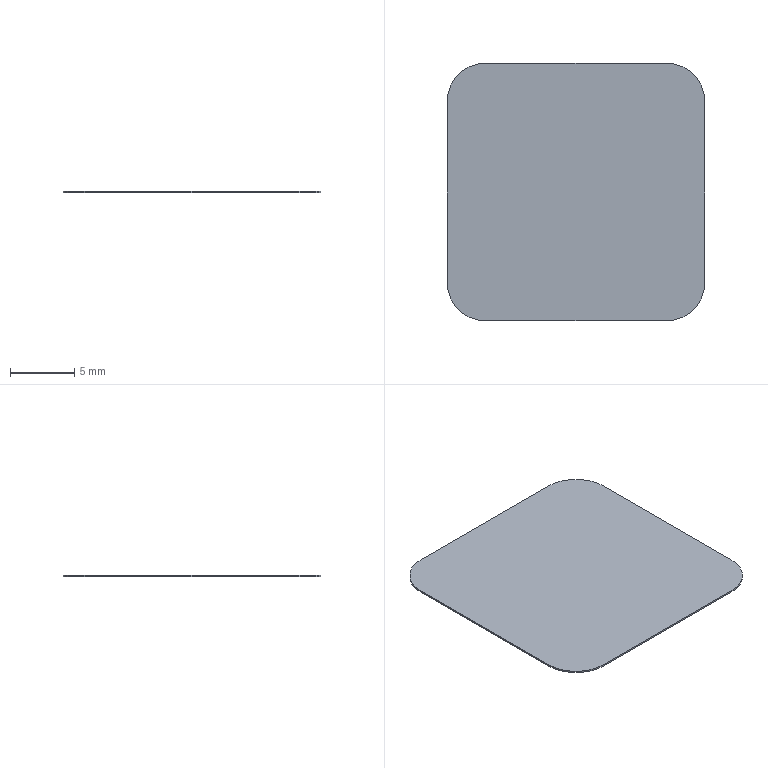Part | STEP file | 68423252 | 1 solid | 10 faces | box 20 x 20 x 0.125 mm | volume 49.034 mm3 | plane 6 | cylinder 4 | commonest cylinder face diameters 6 x4
STEP:
#1=CARTESIAN_POINT('',(0.,0.,0.));
#2=DIRECTION('',(0.,0.,1.));
#3=DIRECTION('',(1.,0.,0.));
#4=AXIS2_PLACEMENT_3D('',#1,#2,#3);
#5=CARTESIAN_POINT('',(-10.,17.,0.));
#6=VERTEX_POINT('',#5);
#7=CARTESIAN_POINT('',(-7.,20.,0.));
#8=VERTEX_POINT('',#7);
#9=CARTESIAN_POINT('',(-7.,17.,0.));
#10=DIRECTION('',(0.,0.,-1.));
#11=DIRECTION('',(-1.,0.,0.));
#12=AXIS2_PLACEMENT_3D('',#9,#10,#11);
#13=CIRCLE('',#12,3.);
#14=CARTESIAN_POINT('',(0.,0.,0.));
#15=DIRECTION('',(0.,0.,1.));
#16=DIRECTION('',(1.,0.,0.));
#17=AXIS2_PLACEMENT_3D('',#14,#15,#16);
#18=PLANE('',#17);
#19=CARTESIAN_POINT('',(-10.,17.));
#20=CARTESIAN_POINT('',(-10.,22.196));
#21=CARTESIAN_POINT('',(-5.5,19.598));
#22=CARTESIAN_POINT('',(-1.,17.));
#23=CARTESIAN_POINT('',(-5.5,14.402));
#24=CARTESIAN_POINT('',(-10.,11.804));
#25=CARTESIAN_POINT('',(-10.,17.));
#26=(BOUNDED_CURVE()B_SPLINE_CURVE(2,(#19,#20,#21,#22,#23,#24,#25),.UNSPECIFIED.,.T.,.F.)B_SPLINE_CURVE_WITH_KNOTS((1,2,2,2,2,1),(-2.094,0.,2.094,4.189,6.283,8.378),.UNSPECIFIED.)CURVE()GEOMETRIC_REPRESENTATION_ITEM()RATIONAL_B_SPLINE_CURVE((1.,0.5,1.,0.5,1.,0.5,1.))REPRESENTATION_ITEM(''));
#27=(GEOMETRIC_REPRESENTATION_CONTEXT(2)PARAMETRIC_REPRESENTATION_CONTEXT()REPRESENTATION_CONTEXT('',''));
#28=DEFINITIONAL_REPRESENTATION('',(#26),#27);
#29=PCURVE('',#18,#28);
#30=CARTESIAN_POINT('',(-7.,17.,0.202));
#31=DIRECTION('',(0.,0.,-1.));
#32=DIRECTION('',(-1.,0.,0.));
#33=AXIS2_PLACEMENT_3D('',#30,#31,#32);
#34=CYLINDRICAL_SURFACE('',#33,3.);
#35=CARTESIAN_POINT('',(0.,0.202));
#36=DIRECTION('',(1.,0.));
#37=VECTOR('',#36,1.);
#38=LINE('',#35,#37);
#39=(GEOMETRIC_REPRESENTATION_CONTEXT(2)PARAMETRIC_REPRESENTATION_CONTEXT()REPRESENTATION_CONTEXT('',''));
#40=DEFINITIONAL_REPRESENTATION('',(#38),#39);
#41=PCURVE('',#34,#40);
#42=SURFACE_CURVE('',#13,(#29,#41),.PCURVE_S1.);
#43=EDGE_CURVE('',#6,#8,#42,.T.);
#44=ORIENTED_EDGE('',*,*,#43,.F.);
#45=CARTESIAN_POINT('',(-10.,3.,0.));
#46=VERTEX_POINT('',#45);
#47=CARTESIAN_POINT('',(-10.,17.,0.));
#48=DIRECTION('',(0.,-1.,0.));
#49=VECTOR('',#48,1.);
#50=LINE('',#47,#49);
#51=CARTESIAN_POINT('',(-10.,17.));
#52=DIRECTION('',(0.,-1.));
#53=VECTOR('',#52,1.);
#54=LINE('',#51,#53);
#55=(GEOMETRIC_REPRESENTATION_CONTEXT(2)PARAMETRIC_REPRESENTATION_CONTEXT()REPRESENTATION_CONTEXT('',''));
#56=DEFINITIONAL_REPRESENTATION('',(#54),#55);
#57=PCURVE('',#18,#56);
#58=CARTESIAN_POINT('',(-10.,20.,0.));
#59=DIRECTION('',(-1.,0.,0.));
#60=DIRECTION('',(0.,-1.,0.));
#61=AXIS2_PLACEMENT_3D('',#58,#59,#60);
#62=PLANE('',#61);
#63=CARTESIAN_POINT('',(3.,0.));
#64=DIRECTION('',(1.,0.));
#65=VECTOR('',#64,1.);
#66=LINE('',#63,#65);
#67=(GEOMETRIC_REPRESENTATION_CONTEXT(2)PARAMETRIC_REPRESENTATION_CONTEXT()REPRESENTATION_CONTEXT('',''));
#68=DEFINITIONAL_REPRESENTATION('',(#66),#67);
#69=PCURVE('',#62,#68);
#70=SURFACE_CURVE('',#50,(#57,#69),.PCURVE_S1.);
#71=EDGE_CURVE('',#6,#46,#70,.T.);
#72=ORIENTED_EDGE('',*,*,#71,.T.);
#73=CARTESIAN_POINT('',(-7.,0.,0.));
#74=VERTEX_POINT('',#73);
#75=CARTESIAN_POINT('',(-7.,3.,0.));
#76=DIRECTION('',(0.,0.,-1.));
#77=DIRECTION('',(0.,-1.,0.));
#78=AXIS2_PLACEMENT_3D('',#75,#76,#77);
#79=CIRCLE('',#78,3.);
#80=CARTESIAN_POINT('',(-7.,0.));
#81=CARTESIAN_POINT('',(-12.196,0.));
#82=CARTESIAN_POINT('',(-9.598,4.5));
#83=CARTESIAN_POINT('',(-7.,9.));
#84=CARTESIAN_POINT('',(-4.402,4.5));
#85=CARTESIAN_POINT('',(-1.804,0.));
#86=CARTESIAN_POINT('',(-7.,0.));
#87=(BOUNDED_CURVE()B_SPLINE_CURVE(2,(#80,#81,#82,#83,#84,#85,#86),.UNSPECIFIED.,.T.,.F.)B_SPLINE_CURVE_WITH_KNOTS((1,2,2,2,2,1),(-2.094,0.,2.094,4.189,6.283,8.378),.UNSPECIFIED.)CURVE()GEOMETRIC_REPRESENTATION_ITEM()RATIONAL_B_SPLINE_CURVE((1.,0.5,1.,0.5,1.,0.5,1.))REPRESENTATION_ITEM(''));
#88=(GEOMETRIC_REPRESENTATION_CONTEXT(2)PARAMETRIC_REPRESENTATION_CONTEXT()REPRESENTATION_CONTEXT('',''));
#89=DEFINITIONAL_REPRESENTATION('',(#87),#88);
#90=PCURVE('',#18,#89);
#91=CARTESIAN_POINT('',(-7.,3.,-0.06577));
#92=DIRECTION('',(0.,0.,1.));
#93=DIRECTION('',(-1.,0.,0.));
#94=AXIS2_PLACEMENT_3D('',#91,#92,#93);
#95=CYLINDRICAL_SURFACE('',#94,3.);
#96=CARTESIAN_POINT('',(1.571,0.06577));
#97=DIRECTION('',(-1.,0.));
#98=VECTOR('',#97,1.);
#99=LINE('',#96,#98);
#100=(GEOMETRIC_REPRESENTATION_CONTEXT(2)PARAMETRIC_REPRESENTATION_CONTEXT()REPRESENTATION_CONTEXT('',''));
#101=DEFINITIONAL_REPRESENTATION('',(#99),#100);
#102=PCURVE('',#95,#101);
#103=SURFACE_CURVE('',#79,(#90,#102),.PCURVE_S1.);
#104=EDGE_CURVE('',#74,#46,#103,.T.);
#105=ORIENTED_EDGE('',*,*,#104,.F.);
#106=CARTESIAN_POINT('',(7.,0.,0.));
#107=VERTEX_POINT('',#106);
#108=CARTESIAN_POINT('',(-7.,0.,0.));
#109=DIRECTION('',(1.,0.,0.));
#110=VECTOR('',#109,1.);
#111=LINE('',#108,#110);
#112=CARTESIAN_POINT('',(-7.,0.));
#113=DIRECTION('',(1.,0.));
#114=VECTOR('',#113,1.);
#115=LINE('',#112,#114);
#116=(GEOMETRIC_REPRESENTATION_CONTEXT(2)PARAMETRIC_REPRESENTATION_CONTEXT()REPRESENTATION_CONTEXT('',''));
#117=DEFINITIONAL_REPRESENTATION('',(#115),#116);
#118=PCURVE('',#18,#117);
#119=CARTESIAN_POINT('',(10.,0.,0.125));
#120=DIRECTION('',(0.,1.,0.));
#121=DIRECTION('',(-1.,0.,0.));
#122=AXIS2_PLACEMENT_3D('',#119,#120,#121);
#123=PLANE('',#122);
#124=CARTESIAN_POINT('',(17.,-0.125));
#125=DIRECTION('',(-1.,0.));
#126=VECTOR('',#125,1.);
#127=LINE('',#124,#126);
#128=(GEOMETRIC_REPRESENTATION_CONTEXT(2)PARAMETRIC_REPRESENTATION_CONTEXT()REPRESENTATION_CONTEXT('',''));
#129=DEFINITIONAL_REPRESENTATION('',(#127),#128);
#130=PCURVE('',#123,#129);
#131=SURFACE_CURVE('',#111,(#118,#130),.PCURVE_S1.);
#132=EDGE_CURVE('',#74,#107,#131,.T.);
#133=ORIENTED_EDGE('',*,*,#132,.T.);
#134=CARTESIAN_POINT('',(10.,3.,0.));
#135=VERTEX_POINT('',#134);
#136=CARTESIAN_POINT('',(7.,3.,0.));
#137=DIRECTION('',(0.,0.,-1.));
#138=DIRECTION('',(1.,0.,0.));
#139=AXIS2_PLACEMENT_3D('',#136,#137,#138);
#140=CIRCLE('',#139,3.);
#141=CARTESIAN_POINT('',(10.,3.));
#142=CARTESIAN_POINT('',(10.,-2.196));
#143=CARTESIAN_POINT('',(5.5,0.4019));
#144=CARTESIAN_POINT('',(1.,3.));
#145=CARTESIAN_POINT('',(5.5,5.598));
#146=CARTESIAN_POINT('',(10.,8.196));
#147=CARTESIAN_POINT('',(10.,3.));
#148=(BOUNDED_CURVE()B_SPLINE_CURVE(2,(#141,#142,#143,#144,#145,#146,#147),.UNSPECIFIED.,.T.,.F.)B_SPLINE_CURVE_WITH_KNOTS((1,2,2,2,2,1),(-2.094,0.,2.094,4.189,6.283,8.378),.UNSPECIFIED.)CURVE()GEOMETRIC_REPRESENTATION_ITEM()RATIONAL_B_SPLINE_CURVE((1.,0.5,1.,0.5,1.,0.5,1.))REPRESENTATION_ITEM(''));
#149=(GEOMETRIC_REPRESENTATION_CONTEXT(2)PARAMETRIC_REPRESENTATION_CONTEXT()REPRESENTATION_CONTEXT('',''));
#150=DEFINITIONAL_REPRESENTATION('',(#148),#149);
#151=PCURVE('',#18,#150);
#152=CARTESIAN_POINT('',(7.,3.,0.202));
#153=DIRECTION('',(0.,0.,-1.));
#154=DIRECTION('',(1.,0.,0.));
#155=AXIS2_PLACEMENT_3D('',#152,#153,#154);
#156=CYLINDRICAL_SURFACE('',#155,3.);
#157=CARTESIAN_POINT('',(0.,0.202));
#158=DIRECTION('',(1.,0.));
#159=VECTOR('',#158,1.);
#160=LINE('',#157,#159);
#161=(GEOMETRIC_REPRESENTATION_CONTEXT(2)PARAMETRIC_REPRESENTATION_CONTEXT()REPRESENTATION_CONTEXT('',''));
#162=DEFINITIONAL_REPRESENTATION('',(#160),#161);
#163=PCURVE('',#156,#162);
#164=SURFACE_CURVE('',#140,(#151,#163),.PCURVE_S1.);
#165=EDGE_CURVE('',#135,#107,#164,.T.);
#166=ORIENTED_EDGE('',*,*,#165,.F.);
#167=CARTESIAN_POINT('',(10.,17.,0.));
#168=VERTEX_POINT('',#167);
#169=CARTESIAN_POINT('',(10.,3.,0.));
#170=DIRECTION('',(0.,1.,0.));
#171=VECTOR('',#170,1.);
#172=LINE('',#169,#171);
#173=CARTESIAN_POINT('',(10.,3.));
#174=DIRECTION('',(0.,1.));
#175=VECTOR('',#174,1.);
#176=LINE('',#173,#175);
#177=(GEOMETRIC_REPRESENTATION_CONTEXT(2)PARAMETRIC_REPRESENTATION_CONTEXT()REPRESENTATION_CONTEXT('',''));
#178=DEFINITIONAL_REPRESENTATION('',(#176),#177);
#179=PCURVE('',#18,#178);
#180=CARTESIAN_POINT('',(10.,-20.,0.));
#181=DIRECTION('',(1.,0.,0.));
#182=DIRECTION('',(0.,1.,0.));
#183=AXIS2_PLACEMENT_3D('',#180,#181,#182);
#184=PLANE('',#183);
#185=CARTESIAN_POINT('',(23.,0.));
#186=DIRECTION('',(1.,0.));
#187=VECTOR('',#186,1.);
#188=LINE('',#185,#187);
#189=(GEOMETRIC_REPRESENTATION_CONTEXT(2)PARAMETRIC_REPRESENTATION_CONTEXT()REPRESENTATION_CONTEXT('',''));
#190=DEFINITIONAL_REPRESENTATION('',(#188),#189);
#191=PCURVE('',#184,#190);
#192=SURFACE_CURVE('',#172,(#179,#191),.PCURVE_S1.);
#193=EDGE_CURVE('',#135,#168,#192,.T.);
#194=ORIENTED_EDGE('',*,*,#193,.T.);
#195=CARTESIAN_POINT('',(7.,20.,0.));
#196=VERTEX_POINT('',#195);
#197=CARTESIAN_POINT('',(7.,17.,0.));
#198=DIRECTION('',(0.,0.,-1.));
#199=DIRECTION('',(0.,1.,0.));
#200=AXIS2_PLACEMENT_3D('',#197,#198,#199);
#201=CIRCLE('',#200,3.);
#202=CARTESIAN_POINT('',(7.,20.));
#203=CARTESIAN_POINT('',(12.196,20.));
#204=CARTESIAN_POINT('',(9.598,15.5));
#205=CARTESIAN_POINT('',(7.,11.));
#206=CARTESIAN_POINT('',(4.402,15.5));
#207=CARTESIAN_POINT('',(1.804,20.));
#208=CARTESIAN_POINT('',(7.,20.));
#209=(BOUNDED_CURVE()B_SPLINE_CURVE(2,(#202,#203,#204,#205,#206,#207,#208),.UNSPECIFIED.,.T.,.F.)B_SPLINE_CURVE_WITH_KNOTS((1,2,2,2,2,1),(-2.094,0.,2.094,4.189,6.283,8.378),.UNSPECIFIED.)CURVE()GEOMETRIC_REPRESENTATION_ITEM()RATIONAL_B_SPLINE_CURVE((1.,0.5,1.,0.5,1.,0.5,1.))REPRESENTATION_ITEM(''));
#210=(GEOMETRIC_REPRESENTATION_CONTEXT(2)PARAMETRIC_REPRESENTATION_CONTEXT()REPRESENTATION_CONTEXT('',''));
#211=DEFINITIONAL_REPRESENTATION('',(#209),#210);
#212=PCURVE('',#18,#211);
#213=CARTESIAN_POINT('',(7.,17.,0.202));
#214=DIRECTION('',(0.,0.,-1.));
#215=DIRECTION('',(0.,1.,0.));
#216=AXIS2_PLACEMENT_3D('',#213,#214,#215);
#217=CYLINDRICAL_SURFACE('',#216,3.);
#218=CARTESIAN_POINT('',(0.,0.202));
#219=DIRECTION('',(1.,0.));
#220=VECTOR('',#219,1.);
#221=LINE('',#218,#220);
#222=(GEOMETRIC_REPRESENTATION_CONTEXT(2)PARAMETRIC_REPRESENTATION_CONTEXT()REPRESENTATION_CONTEXT('',''));
#223=DEFINITIONAL_REPRESENTATION('',(#221),#222);
#224=PCURVE('',#217,#223);
#225=SURFACE_CURVE('',#201,(#212,#224),.PCURVE_S1.);
#226=EDGE_CURVE('',#196,#168,#225,.T.);
#227=ORIENTED_EDGE('',*,*,#226,.F.);
#228=CARTESIAN_POINT('',(7.,20.,0.));
#229=DIRECTION('',(-1.,0.,0.));
#230=VECTOR('',#229,1.);
#231=LINE('',#228,#230);
#232=CARTESIAN_POINT('',(7.,20.));
#233=DIRECTION('',(-1.,0.));
#234=VECTOR('',#233,1.);
#235=LINE('',#232,#234);
#236=(GEOMETRIC_REPRESENTATION_CONTEXT(2)PARAMETRIC_REPRESENTATION_CONTEXT()REPRESENTATION_CONTEXT('',''));
#237=DEFINITIONAL_REPRESENTATION('',(#235),#236);
#238=PCURVE('',#18,#237);
#239=CARTESIAN_POINT('',(10.,20.,0.));
#240=DIRECTION('',(0.,1.,0.));
#241=DIRECTION('',(-1.,0.,0.));
#242=AXIS2_PLACEMENT_3D('',#239,#240,#241);
#243=PLANE('',#242);
#244=CARTESIAN_POINT('',(3.,0.));
#245=DIRECTION('',(1.,0.));
#246=VECTOR('',#245,1.);
#247=LINE('',#244,#246);
#248=(GEOMETRIC_REPRESENTATION_CONTEXT(2)PARAMETRIC_REPRESENTATION_CONTEXT()REPRESENTATION_CONTEXT('',''));
#249=DEFINITIONAL_REPRESENTATION('',(#247),#248);
#250=PCURVE('',#243,#249);
#251=SURFACE_CURVE('',#231,(#238,#250),.PCURVE_S1.);
#252=EDGE_CURVE('',#196,#8,#251,.T.);
#253=ORIENTED_EDGE('',*,*,#252,.T.);
#254=EDGE_LOOP('',(#44,#72,#105,#133,#166,#194,#227,#253));
#255=FACE_BOUND('',#254,.F.);
#256=ADVANCED_FACE('',(#255),#18,.F.);
#257=ORIENTED_EDGE('',*,*,#43,.F.);
#258=CARTESIAN_POINT('',(-10.,17.,0.125));
#259=VERTEX_POINT('',#258);
#260=CARTESIAN_POINT('',(-10.,17.,0.125));
#261=DIRECTION('',(0.,0.,-1.));
#262=VECTOR('',#261,1.);
#263=LINE('',#260,#262);
#264=CARTESIAN_POINT('',(0.,0.07697));
#265=DIRECTION('',(0.,1.));
#266=VECTOR('',#265,1.);
#267=LINE('',#264,#266);
#268=(GEOMETRIC_REPRESENTATION_CONTEXT(2)PARAMETRIC_REPRESENTATION_CONTEXT()REPRESENTATION_CONTEXT('',''));
#269=DEFINITIONAL_REPRESENTATION('',(#267),#268);
#270=PCURVE('',#34,#269);
#271=CARTESIAN_POINT('',(3.,0.125));
#272=DIRECTION('',(0.,-1.));
#273=VECTOR('',#272,1.);
#274=LINE('',#271,#273);
#275=(GEOMETRIC_REPRESENTATION_CONTEXT(2)PARAMETRIC_REPRESENTATION_CONTEXT()REPRESENTATION_CONTEXT('',''));
#276=DEFINITIONAL_REPRESENTATION('',(#274),#275);
#277=PCURVE('',#62,#276);
#278=SURFACE_CURVE('',#263,(#270,#277),.PCURVE_S1.);
#279=EDGE_CURVE('',#259,#6,#278,.T.);
#280=ORIENTED_EDGE('',*,*,#279,.F.);
#281=CARTESIAN_POINT('',(-7.,20.,0.125));
#282=VERTEX_POINT('',#281);
#283=CARTESIAN_POINT('',(-7.,17.,0.125));
#284=DIRECTION('',(0.,0.,1.));
#285=DIRECTION('',(0.,1.,0.));
#286=AXIS2_PLACEMENT_3D('',#283,#284,#285);
#287=CIRCLE('',#286,3.);
#288=CARTESIAN_POINT('',(1.571,0.07697));
#289=DIRECTION('',(-1.,0.));
#290=VECTOR('',#289,1.);
#291=LINE('',#288,#290);
#292=(GEOMETRIC_REPRESENTATION_CONTEXT(2)PARAMETRIC_REPRESENTATION_CONTEXT()REPRESENTATION_CONTEXT('',''));
#293=DEFINITIONAL_REPRESENTATION('',(#291),#292);
#294=PCURVE('',#34,#293);
#295=CARTESIAN_POINT('',(0.,0.,0.125));
#296=DIRECTION('',(0.,0.,1.));
#297=DIRECTION('',(1.,0.,0.));
#298=AXIS2_PLACEMENT_3D('',#295,#296,#297);
#299=PLANE('',#298);
#300=CARTESIAN_POINT('',(-7.,17.));
#301=DIRECTION('',(0.,1.));
#302=AXIS2_PLACEMENT_2D('',#300,#301);
#303=CIRCLE('',#302,3.);
#304=(GEOMETRIC_REPRESENTATION_CONTEXT(2)PARAMETRIC_REPRESENTATION_CONTEXT()REPRESENTATION_CONTEXT('',''));
#305=DEFINITIONAL_REPRESENTATION('',(#303),#304);
#306=PCURVE('',#299,#305);
#307=SURFACE_CURVE('',#287,(#294,#306),.PCURVE_S1.);
#308=EDGE_CURVE('',#282,#259,#307,.T.);
#309=ORIENTED_EDGE('',*,*,#308,.F.);
#310=CARTESIAN_POINT('',(-7.,20.,0.125));
#311=DIRECTION('',(0.,0.,-1.));
#312=VECTOR('',#311,1.);
#313=LINE('',#310,#312);
#314=CARTESIAN_POINT('',(1.571,0.07697));
#315=DIRECTION('',(0.,1.));
#316=VECTOR('',#315,1.);
#317=LINE('',#314,#316);
#318=(GEOMETRIC_REPRESENTATION_CONTEXT(2)PARAMETRIC_REPRESENTATION_CONTEXT()REPRESENTATION_CONTEXT('',''));
#319=DEFINITIONAL_REPRESENTATION('',(#317),#318);
#320=PCURVE('',#34,#319);
#321=CARTESIAN_POINT('',(17.,0.125));
#322=DIRECTION('',(0.,-1.));
#323=VECTOR('',#322,1.);
#324=LINE('',#321,#323);
#325=(GEOMETRIC_REPRESENTATION_CONTEXT(2)PARAMETRIC_REPRESENTATION_CONTEXT()REPRESENTATION_CONTEXT('',''));
#326=DEFINITIONAL_REPRESENTATION('',(#324),#325);
#327=PCURVE('',#243,#326);
#328=SURFACE_CURVE('',#313,(#320,#327),.PCURVE_S1.);
#329=EDGE_CURVE('',#282,#8,#328,.T.);
#330=ORIENTED_EDGE('',*,*,#329,.T.);
#331=EDGE_LOOP('',(#257,#280,#309,#330));
#332=FACE_BOUND('',#331,.T.);
#333=ADVANCED_FACE('',(#332),#34,.T.);
#334=ORIENTED_EDGE('',*,*,#329,.T.);
#335=ORIENTED_EDGE('',*,*,#252,.F.);
#336=CARTESIAN_POINT('',(7.,20.,0.125));
#337=VERTEX_POINT('',#336);
#338=CARTESIAN_POINT('',(7.,20.,0.125));
#339=DIRECTION('',(0.,0.,-1.));
#340=VECTOR('',#339,1.);
#341=LINE('',#338,#340);
#342=CARTESIAN_POINT('',(3.,0.125));
#343=DIRECTION('',(0.,-1.));
#344=VECTOR('',#343,1.);
#345=LINE('',#342,#344);
#346=(GEOMETRIC_REPRESENTATION_CONTEXT(2)PARAMETRIC_REPRESENTATION_CONTEXT()REPRESENTATION_CONTEXT('',''));
#347=DEFINITIONAL_REPRESENTATION('',(#345),#346);
#348=PCURVE('',#243,#347);
#349=CARTESIAN_POINT('',(0.,0.07697));
#350=DIRECTION('',(0.,1.));
#351=VECTOR('',#350,1.);
#352=LINE('',#349,#351);
#353=(GEOMETRIC_REPRESENTATION_CONTEXT(2)PARAMETRIC_REPRESENTATION_CONTEXT()REPRESENTATION_CONTEXT('',''));
#354=DEFINITIONAL_REPRESENTATION('',(#352),#353);
#355=PCURVE('',#217,#354);
#356=SURFACE_CURVE('',#341,(#348,#355),.PCURVE_S1.);
#357=EDGE_CURVE('',#337,#196,#356,.T.);
#358=ORIENTED_EDGE('',*,*,#357,.F.);
#359=CARTESIAN_POINT('',(7.,20.,0.125));
#360=DIRECTION('',(-1.,0.,0.));
#361=VECTOR('',#360,1.);
#362=LINE('',#359,#361);
#363=CARTESIAN_POINT('',(3.,0.125));
#364=DIRECTION('',(1.,0.));
#365=VECTOR('',#364,1.);
#366=LINE('',#363,#365);
#367=(GEOMETRIC_REPRESENTATION_CONTEXT(2)PARAMETRIC_REPRESENTATION_CONTEXT()REPRESENTATION_CONTEXT('',''));
#368=DEFINITIONAL_REPRESENTATION('',(#366),#367);
#369=PCURVE('',#243,#368);
#370=CARTESIAN_POINT('',(7.,20.));
#371=DIRECTION('',(-1.,0.));
#372=VECTOR('',#371,1.);
#373=LINE('',#370,#372);
#374=(GEOMETRIC_REPRESENTATION_CONTEXT(2)PARAMETRIC_REPRESENTATION_CONTEXT()REPRESENTATION_CONTEXT('',''));
#375=DEFINITIONAL_REPRESENTATION('',(#373),#374);
#376=PCURVE('',#299,#375);
#377=SURFACE_CURVE('',#362,(#369,#376),.PCURVE_S1.);
#378=EDGE_CURVE('',#337,#282,#377,.T.);
#379=ORIENTED_EDGE('',*,*,#378,.T.);
#380=EDGE_LOOP('',(#334,#335,#358,#379));
#381=FACE_BOUND('',#380,.F.);
#382=ADVANCED_FACE('',(#381),#243,.T.);
#383=ORIENTED_EDGE('',*,*,#226,.F.);
#384=ORIENTED_EDGE('',*,*,#357,.F.);
#385=CARTESIAN_POINT('',(10.,17.,0.125));
#386=VERTEX_POINT('',#385);
#387=CARTESIAN_POINT('',(7.,17.,0.125));
#388=DIRECTION('',(0.,0.,1.));
#389=DIRECTION('',(1.,0.,0.));
#390=AXIS2_PLACEMENT_3D('',#387,#388,#389);
#391=CIRCLE('',#390,3.);
#392=CARTESIAN_POINT('',(1.571,0.07697));
#393=DIRECTION('',(-1.,0.));
#394=VECTOR('',#393,1.);
#395=LINE('',#392,#394);
#396=(GEOMETRIC_REPRESENTATION_CONTEXT(2)PARAMETRIC_REPRESENTATION_CONTEXT()REPRESENTATION_CONTEXT('',''));
#397=DEFINITIONAL_REPRESENTATION('',(#395),#396);
#398=PCURVE('',#217,#397);
#399=CARTESIAN_POINT('',(7.,17.));
#400=DIRECTION('',(1.,0.));
#401=AXIS2_PLACEMENT_2D('',#399,#400);
#402=CIRCLE('',#401,3.);
#403=(GEOMETRIC_REPRESENTATION_CONTEXT(2)PARAMETRIC_REPRESENTATION_CONTEXT()REPRESENTATION_CONTEXT('',''));
#404=DEFINITIONAL_REPRESENTATION('',(#402),#403);
#405=PCURVE('',#299,#404);
#406=SURFACE_CURVE('',#391,(#398,#405),.PCURVE_S1.);
#407=EDGE_CURVE('',#386,#337,#406,.T.);
#408=ORIENTED_EDGE('',*,*,#407,.F.);
#409=CARTESIAN_POINT('',(10.,17.,0.125));
#410=DIRECTION('',(0.,0.,-1.));
#411=VECTOR('',#410,1.);
#412=LINE('',#409,#411);
#413=CARTESIAN_POINT('',(1.571,0.07697));
#414=DIRECTION('',(0.,1.));
#415=VECTOR('',#414,1.);
#416=LINE('',#413,#415);
#417=(GEOMETRIC_REPRESENTATION_CONTEXT(2)PARAMETRIC_REPRESENTATION_CONTEXT()REPRESENTATION_CONTEXT('',''));
#418=DEFINITIONAL_REPRESENTATION('',(#416),#417);
#419=PCURVE('',#217,#418);
#420=CARTESIAN_POINT('',(37.,0.125));
#421=DIRECTION('',(0.,-1.));
#422=VECTOR('',#421,1.);
#423=LINE('',#420,#422);
#424=(GEOMETRIC_REPRESENTATION_CONTEXT(2)PARAMETRIC_REPRESENTATION_CONTEXT()REPRESENTATION_CONTEXT('',''));
#425=DEFINITIONAL_REPRESENTATION('',(#423),#424);
#426=PCURVE('',#184,#425);
#427=SURFACE_CURVE('',#412,(#419,#426),.PCURVE_S1.);
#428=EDGE_CURVE('',#386,#168,#427,.T.);
#429=ORIENTED_EDGE('',*,*,#428,.T.);
#430=EDGE_LOOP('',(#383,#384,#408,#429));
#431=FACE_BOUND('',#430,.T.);
#432=ADVANCED_FACE('',(#431),#217,.T.);
#433=ORIENTED_EDGE('',*,*,#428,.T.);
#434=ORIENTED_EDGE('',*,*,#193,.F.);
#435=CARTESIAN_POINT('',(10.,3.,0.125));
#436=VERTEX_POINT('',#435);
#437=CARTESIAN_POINT('',(10.,3.,0.125));
#438=DIRECTION('',(0.,0.,-1.));
#439=VECTOR('',#438,1.);
#440=LINE('',#437,#439);
#441=CARTESIAN_POINT('',(23.,0.125));
#442=DIRECTION('',(0.,-1.));
#443=VECTOR('',#442,1.);
#444=LINE('',#441,#443);
#445=(GEOMETRIC_REPRESENTATION_CONTEXT(2)PARAMETRIC_REPRESENTATION_CONTEXT()REPRESENTATION_CONTEXT('',''));
#446=DEFINITIONAL_REPRESENTATION('',(#444),#445);
#447=PCURVE('',#184,#446);
#448=CARTESIAN_POINT('',(0.,0.07697));
#449=DIRECTION('',(0.,1.));
#450=VECTOR('',#449,1.);
#451=LINE('',#448,#450);
#452=(GEOMETRIC_REPRESENTATION_CONTEXT(2)PARAMETRIC_REPRESENTATION_CONTEXT()REPRESENTATION_CONTEXT('',''));
#453=DEFINITIONAL_REPRESENTATION('',(#451),#452);
#454=PCURVE('',#156,#453);
#455=SURFACE_CURVE('',#440,(#447,#454),.PCURVE_S1.);
#456=EDGE_CURVE('',#436,#135,#455,.T.);
#457=ORIENTED_EDGE('',*,*,#456,.F.);
#458=CARTESIAN_POINT('',(10.,3.,0.125));
#459=DIRECTION('',(0.,1.,0.));
#460=VECTOR('',#459,1.);
#461=LINE('',#458,#460);
#462=CARTESIAN_POINT('',(23.,0.125));
#463=DIRECTION('',(1.,0.));
#464=VECTOR('',#463,1.);
#465=LINE('',#462,#464);
#466=(GEOMETRIC_REPRESENTATION_CONTEXT(2)PARAMETRIC_REPRESENTATION_CONTEXT()REPRESENTATION_CONTEXT('',''));
#467=DEFINITIONAL_REPRESENTATION('',(#465),#466);
#468=PCURVE('',#184,#467);
#469=CARTESIAN_POINT('',(10.,3.));
#470=DIRECTION('',(0.,1.));
#471=VECTOR('',#470,1.);
#472=LINE('',#469,#471);
#473=(GEOMETRIC_REPRESENTATION_CONTEXT(2)PARAMETRIC_REPRESENTATION_CONTEXT()REPRESENTATION_CONTEXT('',''));
#474=DEFINITIONAL_REPRESENTATION('',(#472),#473);
#475=PCURVE('',#299,#474);
#476=SURFACE_CURVE('',#461,(#468,#475),.PCURVE_S1.);
#477=EDGE_CURVE('',#436,#386,#476,.T.);
#478=ORIENTED_EDGE('',*,*,#477,.T.);
#479=EDGE_LOOP('',(#433,#434,#457,#478));
#480=FACE_BOUND('',#479,.F.);
#481=ADVANCED_FACE('',(#480),#184,.T.);
#482=ORIENTED_EDGE('',*,*,#165,.F.);
#483=ORIENTED_EDGE('',*,*,#456,.F.);
#484=CARTESIAN_POINT('',(7.,0.,0.125));
#485=VERTEX_POINT('',#484);
#486=CARTESIAN_POINT('',(7.,3.,0.125));
#487=DIRECTION('',(0.,0.,1.));
#488=DIRECTION('',(0.,-1.,0.));
#489=AXIS2_PLACEMENT_3D('',#486,#487,#488);
#490=CIRCLE('',#489,3.);
#491=CARTESIAN_POINT('',(1.571,0.07697));
#492=DIRECTION('',(-1.,0.));
#493=VECTOR('',#492,1.);
#494=LINE('',#491,#493);
#495=(GEOMETRIC_REPRESENTATION_CONTEXT(2)PARAMETRIC_REPRESENTATION_CONTEXT()REPRESENTATION_CONTEXT('',''));
#496=DEFINITIONAL_REPRESENTATION('',(#494),#495);
#497=PCURVE('',#156,#496);
#498=CARTESIAN_POINT('',(7.,3.));
#499=DIRECTION('',(0.,-1.));
#500=AXIS2_PLACEMENT_2D('',#498,#499);
#501=CIRCLE('',#500,3.);
#502=(GEOMETRIC_REPRESENTATION_CONTEXT(2)PARAMETRIC_REPRESENTATION_CONTEXT()REPRESENTATION_CONTEXT('',''));
#503=DEFINITIONAL_REPRESENTATION('',(#501),#502);
#504=PCURVE('',#299,#503);
#505=SURFACE_CURVE('',#490,(#497,#504),.PCURVE_S1.);
#506=EDGE_CURVE('',#485,#436,#505,.T.);
#507=ORIENTED_EDGE('',*,*,#506,.F.);
#508=CARTESIAN_POINT('',(7.,0.,0.125));
#509=DIRECTION('',(0.,0.,-1.));
#510=VECTOR('',#509,1.);
#511=LINE('',#508,#510);
#512=CARTESIAN_POINT('',(1.571,0.07697));
#513=DIRECTION('',(0.,1.));
#514=VECTOR('',#513,1.);
#515=LINE('',#512,#514);
#516=(GEOMETRIC_REPRESENTATION_CONTEXT(2)PARAMETRIC_REPRESENTATION_CONTEXT()REPRESENTATION_CONTEXT('',''));
#517=DEFINITIONAL_REPRESENTATION('',(#515),#516);
#518=PCURVE('',#156,#517);
#519=CARTESIAN_POINT('',(3.,0.));
#520=DIRECTION('',(0.,-1.));
#521=VECTOR('',#520,1.);
#522=LINE('',#519,#521);
#523=(GEOMETRIC_REPRESENTATION_CONTEXT(2)PARAMETRIC_REPRESENTATION_CONTEXT()REPRESENTATION_CONTEXT('',''));
#524=DEFINITIONAL_REPRESENTATION('',(#522),#523);
#525=PCURVE('',#123,#524);
#526=SURFACE_CURVE('',#511,(#518,#525),.PCURVE_S1.);
#527=EDGE_CURVE('',#485,#107,#526,.T.);
#528=ORIENTED_EDGE('',*,*,#527,.T.);
#529=EDGE_LOOP('',(#482,#483,#507,#528));
#530=FACE_BOUND('',#529,.T.);
#531=ADVANCED_FACE('',(#530),#156,.T.);
#532=CARTESIAN_POINT('',(-7.,0.,0.125));
#533=VERTEX_POINT('',#532);
#534=CARTESIAN_POINT('',(-7.,0.,0.));
#535=DIRECTION('',(0.,0.,1.));
#536=VECTOR('',#535,1.);
#537=LINE('',#534,#536);
#538=CARTESIAN_POINT('',(17.,-0.125));
#539=DIRECTION('',(0.,1.));
#540=VECTOR('',#539,1.);
#541=LINE('',#538,#540);
#542=(GEOMETRIC_REPRESENTATION_CONTEXT(2)PARAMETRIC_REPRESENTATION_CONTEXT()REPRESENTATION_CONTEXT('',''));
#543=DEFINITIONAL_REPRESENTATION('',(#541),#542);
#544=PCURVE('',#123,#543);
#545=CARTESIAN_POINT('',(1.571,0.06577));
#546=DIRECTION('',(0.,1.));
#547=VECTOR('',#546,1.);
#548=LINE('',#545,#547);
#549=(GEOMETRIC_REPRESENTATION_CONTEXT(2)PARAMETRIC_REPRESENTATION_CONTEXT()REPRESENTATION_CONTEXT('',''));
#550=DEFINITIONAL_REPRESENTATION('',(#548),#549);
#551=PCURVE('',#95,#550);
#552=SURFACE_CURVE('',#537,(#544,#551),.PCURVE_S1.);
#553=EDGE_CURVE('',#74,#533,#552,.T.);
#554=ORIENTED_EDGE('',*,*,#553,.T.);
#555=CARTESIAN_POINT('',(-7.,0.,0.125));
#556=DIRECTION('',(1.,0.,0.));
#557=VECTOR('',#556,1.);
#558=LINE('',#555,#557);
#559=CARTESIAN_POINT('',(17.,0.));
#560=DIRECTION('',(-1.,0.));
#561=VECTOR('',#560,1.);
#562=LINE('',#559,#561);
#563=(GEOMETRIC_REPRESENTATION_CONTEXT(2)PARAMETRIC_REPRESENTATION_CONTEXT()REPRESENTATION_CONTEXT('',''));
#564=DEFINITIONAL_REPRESENTATION('',(#562),#563);
#565=PCURVE('',#123,#564);
#566=CARTESIAN_POINT('',(-7.,0.));
#567=DIRECTION('',(1.,0.));
#568=VECTOR('',#567,1.);
#569=LINE('',#566,#568);
#570=(GEOMETRIC_REPRESENTATION_CONTEXT(2)PARAMETRIC_REPRESENTATION_CONTEXT()REPRESENTATION_CONTEXT('',''));
#571=DEFINITIONAL_REPRESENTATION('',(#569),#570);
#572=PCURVE('',#299,#571);
#573=SURFACE_CURVE('',#558,(#565,#572),.PCURVE_S1.);
#574=EDGE_CURVE('',#533,#485,#573,.T.);
#575=ORIENTED_EDGE('',*,*,#574,.T.);
#576=ORIENTED_EDGE('',*,*,#527,.T.);
#577=ORIENTED_EDGE('',*,*,#132,.F.);
#578=EDGE_LOOP('',(#554,#575,#576,#577));
#579=FACE_BOUND('',#578,.F.);
#580=ADVANCED_FACE('',(#579),#123,.F.);
#581=CARTESIAN_POINT('',(-10.,3.,0.125));
#582=VERTEX_POINT('',#581);
#583=CARTESIAN_POINT('',(-7.,3.,0.125));
#584=DIRECTION('',(0.,0.,1.));
#585=DIRECTION('',(-1.,0.,0.));
#586=AXIS2_PLACEMENT_3D('',#583,#584,#585);
#587=CIRCLE('',#586,3.);
#588=CARTESIAN_POINT('',(0.,0.1908));
#589=DIRECTION('',(1.,0.));
#590=VECTOR('',#589,1.);
#591=LINE('',#588,#590);
#592=(GEOMETRIC_REPRESENTATION_CONTEXT(2)PARAMETRIC_REPRESENTATION_CONTEXT()REPRESENTATION_CONTEXT('',''));
#593=DEFINITIONAL_REPRESENTATION('',(#591),#592);
#594=PCURVE('',#95,#593);
#595=CARTESIAN_POINT('',(-7.,3.));
#596=DIRECTION('',(-1.,0.));
#597=AXIS2_PLACEMENT_2D('',#595,#596);
#598=CIRCLE('',#597,3.);
#599=(GEOMETRIC_REPRESENTATION_CONTEXT(2)PARAMETRIC_REPRESENTATION_CONTEXT()REPRESENTATION_CONTEXT('',''));
#600=DEFINITIONAL_REPRESENTATION('',(#598),#599);
#601=PCURVE('',#299,#600);
#602=SURFACE_CURVE('',#587,(#594,#601),.PCURVE_S1.);
#603=EDGE_CURVE('',#582,#533,#602,.T.);
#604=ORIENTED_EDGE('',*,*,#603,.F.);
#605=CARTESIAN_POINT('',(-10.,3.,0.));
#606=DIRECTION('',(0.,0.,1.));
#607=VECTOR('',#606,1.);
#608=LINE('',#605,#607);
#609=CARTESIAN_POINT('',(0.,0.06577));
#610=DIRECTION('',(0.,1.));
#611=VECTOR('',#610,1.);
#612=LINE('',#609,#611);
#613=(GEOMETRIC_REPRESENTATION_CONTEXT(2)PARAMETRIC_REPRESENTATION_CONTEXT()REPRESENTATION_CONTEXT('',''));
#614=DEFINITIONAL_REPRESENTATION('',(#612),#613);
#615=PCURVE('',#95,#614);
#616=CARTESIAN_POINT('',(17.,0.));
#617=DIRECTION('',(0.,1.));
#618=VECTOR('',#617,1.);
#619=LINE('',#616,#618);
#620=(GEOMETRIC_REPRESENTATION_CONTEXT(2)PARAMETRIC_REPRESENTATION_CONTEXT()REPRESENTATION_CONTEXT('',''));
#621=DEFINITIONAL_REPRESENTATION('',(#619),#620);
#622=PCURVE('',#62,#621);
#623=SURFACE_CURVE('',#608,(#615,#622),.PCURVE_S1.);
#624=EDGE_CURVE('',#46,#582,#623,.T.);
#625=ORIENTED_EDGE('',*,*,#624,.F.);
#626=ORIENTED_EDGE('',*,*,#104,.F.);
#627=ORIENTED_EDGE('',*,*,#553,.T.);
#628=EDGE_LOOP('',(#604,#625,#626,#627));
#629=FACE_BOUND('',#628,.T.);
#630=ADVANCED_FACE('',(#629),#95,.T.);
#631=ORIENTED_EDGE('',*,*,#279,.F.);
#632=CARTESIAN_POINT('',(-10.,17.,0.125));
#633=DIRECTION('',(0.,-1.,0.));
#634=VECTOR('',#633,1.);
#635=LINE('',#632,#634);
#636=CARTESIAN_POINT('',(3.,0.125));
#637=DIRECTION('',(1.,0.));
#638=VECTOR('',#637,1.);
#639=LINE('',#636,#638);
#640=(GEOMETRIC_REPRESENTATION_CONTEXT(2)PARAMETRIC_REPRESENTATION_CONTEXT()REPRESENTATION_CONTEXT('',''));
#641=DEFINITIONAL_REPRESENTATION('',(#639),#640);
#642=PCURVE('',#62,#641);
#643=CARTESIAN_POINT('',(-10.,17.));
#644=DIRECTION('',(0.,-1.));
#645=VECTOR('',#644,1.);
#646=LINE('',#643,#645);
#647=(GEOMETRIC_REPRESENTATION_CONTEXT(2)PARAMETRIC_REPRESENTATION_CONTEXT()REPRESENTATION_CONTEXT('',''));
#648=DEFINITIONAL_REPRESENTATION('',(#646),#647);
#649=PCURVE('',#299,#648);
#650=SURFACE_CURVE('',#635,(#642,#649),.PCURVE_S1.);
#651=EDGE_CURVE('',#259,#582,#650,.T.);
#652=ORIENTED_EDGE('',*,*,#651,.T.);
#653=ORIENTED_EDGE('',*,*,#624,.F.);
#654=ORIENTED_EDGE('',*,*,#71,.F.);
#655=EDGE_LOOP('',(#631,#652,#653,#654));
#656=FACE_BOUND('',#655,.F.);
#657=ADVANCED_FACE('',(#656),#62,.T.);
#658=ORIENTED_EDGE('',*,*,#308,.F.);
#659=ORIENTED_EDGE('',*,*,#378,.F.);
#660=ORIENTED_EDGE('',*,*,#407,.F.);
#661=ORIENTED_EDGE('',*,*,#477,.F.);
#662=ORIENTED_EDGE('',*,*,#506,.F.);
#663=ORIENTED_EDGE('',*,*,#574,.F.);
#664=ORIENTED_EDGE('',*,*,#603,.F.);
#665=ORIENTED_EDGE('',*,*,#651,.F.);
#666=EDGE_LOOP('',(#658,#659,#660,#661,#662,#663,#664,#665));
#667=FACE_BOUND('',#666,.F.);
#668=ADVANCED_FACE('',(#667),#299,.T.);
#669=CLOSED_SHELL('',(#256,#333,#382,#432,#481,#531,#580,#630,#657,#668));
#670=MANIFOLD_SOLID_BREP('',#669);
#671=(LENGTH_UNIT()NAMED_UNIT(*)SI_UNIT(.MILLI.,.METRE.));
#672=UNCERTAINTY_MEASURE_WITH_UNIT(LENGTH_MEASURE(0.0000001),#671,'','');
#673=(NAMED_UNIT(*)PLANE_ANGLE_UNIT()SI_UNIT($,.RADIAN.));
#674=(NAMED_UNIT(*)SI_UNIT($,.STERADIAN.)SOLID_ANGLE_UNIT());
#675=(GEOMETRIC_REPRESENTATION_CONTEXT(3)GLOBAL_UNCERTAINTY_ASSIGNED_CONTEXT((#672))GLOBAL_UNIT_ASSIGNED_CONTEXT((#671,#673,#674))REPRESENTATION_CONTEXT('',''));
#676=ADVANCED_BREP_SHAPE_REPRESENTATION('',(#4,#670),#675);